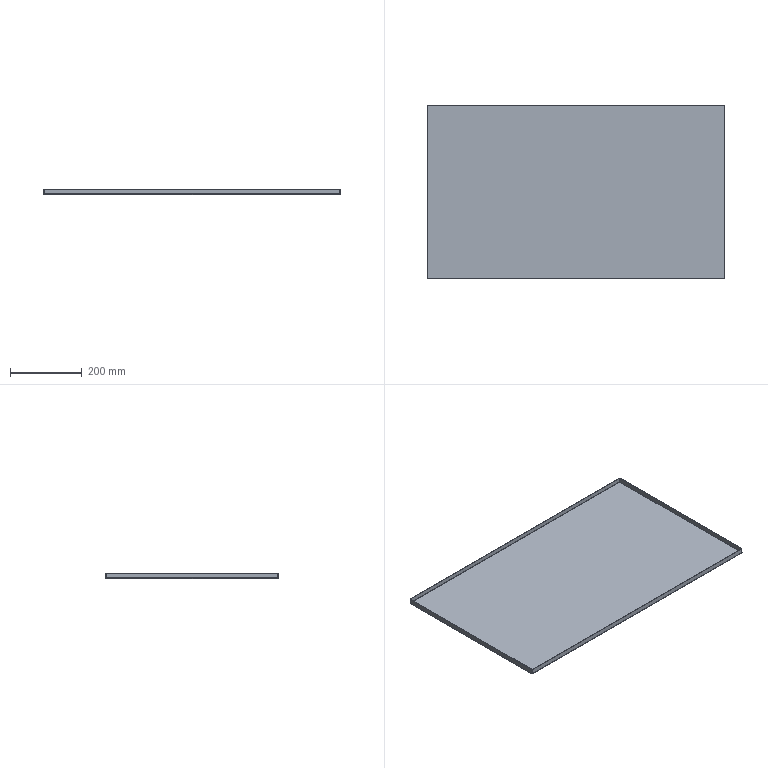Part | SolidWorks | 1 solid | 38 faces | box 830 x 485 x 15 mm | volume 870407 mm3 | plane 22 | spline 8 | cylinder 8 | commonest cylinder face diameters 0.2 x4 4.2 x4
STEP:
#1=CARTESIAN_POINT('',(412.9,-240.4,-2.));
#2=VERTEX_POINT('',#1);
#3=CARTESIAN_POINT('',(-412.9,-240.4,-2.));
#4=VERTEX_POINT('',#3);
#5=CARTESIAN_POINT('',(412.9,-240.4,-2.));
#6=DIRECTION('',(-1.,0.,0.));
#7=VECTOR('',#6,1000.);
#8=LINE('',#5,#7);
#9=EDGE_CURVE('',#2,#4,#8,.T.);
#10=ORIENTED_EDGE('',*,*,#9,.T.);
#11=CARTESIAN_POINT('',(-412.9,240.4,-2.));
#12=VERTEX_POINT('',#11);
#13=CARTESIAN_POINT('',(-412.9,-240.4,-2.));
#14=DIRECTION('',(0.,1.,0.));
#15=VECTOR('',#14,1000.);
#16=LINE('',#13,#15);
#17=EDGE_CURVE('',#4,#12,#16,.T.);
#18=ORIENTED_EDGE('',*,*,#17,.T.);
#19=CARTESIAN_POINT('',(412.9,240.4,-2.));
#20=VERTEX_POINT('',#19);
#21=CARTESIAN_POINT('',(-412.9,240.4,-2.));
#22=DIRECTION('',(1.,0.,0.));
#23=VECTOR('',#22,1000.);
#24=LINE('',#21,#23);
#25=EDGE_CURVE('',#12,#20,#24,.T.);
#26=ORIENTED_EDGE('',*,*,#25,.T.);
#27=CARTESIAN_POINT('',(412.9,240.4,-2.));
#28=DIRECTION('',(0.,-1.,0.));
#29=VECTOR('',#28,1000.);
#30=LINE('',#27,#29);
#31=EDGE_CURVE('',#20,#2,#30,.T.);
#32=ORIENTED_EDGE('',*,*,#31,.T.);
#33=EDGE_LOOP('',(#10,#18,#26,#32));
#34=FACE_OUTER_BOUND('',#33,.T.);
#35=CARTESIAN_POINT('',(0.,0.,-2.));
#36=DIRECTION('',(0.,0.,1.));
#37=DIRECTION('',(1.,0.,0.));
#38=AXIS2_PLACEMENT_3D('',#35,#36,#37);
#39=PLANE('',#38);
#40=ADVANCED_FACE('',(#34),#39,.F.);
#41=CARTESIAN_POINT('',(-412.9,-240.4,0.));
#42=VERTEX_POINT('',#41);
#43=CARTESIAN_POINT('',(-412.9,240.4,0.));
#44=VERTEX_POINT('',#43);
#45=CARTESIAN_POINT('',(-412.9,-240.4,0.));
#46=DIRECTION('',(0.,1.,0.));
#47=VECTOR('',#46,1000.);
#48=LINE('',#45,#47);
#49=EDGE_CURVE('',#42,#44,#48,.T.);
#50=ORIENTED_EDGE('',*,*,#49,.F.);
#51=CARTESIAN_POINT('',(412.9,-240.4,0.));
#52=VERTEX_POINT('',#51);
#53=CARTESIAN_POINT('',(412.9,-240.4,0.));
#54=DIRECTION('',(-1.,0.,0.));
#55=VECTOR('',#54,1000.);
#56=LINE('',#53,#55);
#57=EDGE_CURVE('',#52,#42,#56,.T.);
#58=ORIENTED_EDGE('',*,*,#57,.F.);
#59=CARTESIAN_POINT('',(412.9,240.4,0.));
#60=VERTEX_POINT('',#59);
#61=CARTESIAN_POINT('',(412.9,240.4,0.));
#62=DIRECTION('',(0.,-1.,0.));
#63=VECTOR('',#62,1000.);
#64=LINE('',#61,#63);
#65=EDGE_CURVE('',#60,#52,#64,.T.);
#66=ORIENTED_EDGE('',*,*,#65,.F.);
#67=CARTESIAN_POINT('',(-412.9,240.4,0.));
#68=DIRECTION('',(1.,0.,0.));
#69=VECTOR('',#68,1000.);
#70=LINE('',#67,#69);
#71=EDGE_CURVE('',#44,#60,#70,.T.);
#72=ORIENTED_EDGE('',*,*,#71,.F.);
#73=EDGE_LOOP('',(#50,#58,#66,#72));
#74=FACE_OUTER_BOUND('',#73,.T.);
#75=CARTESIAN_POINT('',(0.,0.,0.));
#76=DIRECTION('',(0.,0.,1.));
#77=DIRECTION('',(1.,0.,0.));
#78=AXIS2_PLACEMENT_3D('',#75,#76,#77);
#79=PLANE('',#78);
#80=ADVANCED_FACE('',(#74),#79,.T.);
#81=CARTESIAN_POINT('',(-415.,239.793,0.1));
#82=VERTEX_POINT('',#81);
#83=CARTESIAN_POINT('',(-413.,239.793,0.1));
#84=VERTEX_POINT('',#83);
#85=CARTESIAN_POINT('',(-413.,239.793,0.1));
#86=DIRECTION('',(1.,0.,0.));
#87=VECTOR('',#86,1000.);
#88=LINE('',#85,#87);
#89=EDGE_CURVE('',#82,#84,#88,.T.);
#90=ORIENTED_EDGE('',*,*,#89,.T.);
#91=CARTESIAN_POINT('',(-412.9,240.4,0.));
#92=CARTESIAN_POINT('',(-412.926,240.299,0.));
#93=CARTESIAN_POINT('',(-412.952,240.198,0.01078));
#94=CARTESIAN_POINT('',(-412.989,239.995,0.0478));
#95=CARTESIAN_POINT('',(-413.,239.894,0.07382));
#96=CARTESIAN_POINT('',(-413.,239.793,0.1));
#97=B_SPLINE_CURVE_WITH_KNOTS('',3,(#91,#92,#93,#94,#95,#96),.UNSPECIFIED.,.F.,.F.,(4,2,4),(0.,0.5,1.),.UNSPECIFIED.);
#98=EDGE_CURVE('',#44,#84,#97,.T.);
#99=ORIENTED_EDGE('',*,*,#98,.F.);
#100=CARTESIAN_POINT('',(-412.9,240.4,0.));
#101=DIRECTION('',(0.,0.,-1.));
#102=VECTOR('',#101,1000.);
#103=LINE('',#100,#102);
#104=EDGE_CURVE('',#44,#12,#103,.T.);
#105=ORIENTED_EDGE('',*,*,#104,.T.);
#106=CARTESIAN_POINT('',(-412.9,240.4,-2.));
#107=CARTESIAN_POINT('',(-413.039,240.374,-2.));
#108=CARTESIAN_POINT('',(-413.175,240.349,-1.986));
#109=CARTESIAN_POINT('',(-413.443,240.299,-1.933));
#110=CARTESIAN_POINT('',(-413.576,240.274,-1.893));
#111=CARTESIAN_POINT('',(-413.831,240.223,-1.787));
#112=CARTESIAN_POINT('',(-413.951,240.198,-1.723));
#113=CARTESIAN_POINT('',(-414.179,240.147,-1.571));
#114=CARTESIAN_POINT('',(-414.287,240.122,-1.482));
#115=CARTESIAN_POINT('',(-414.481,240.071,-1.289));
#116=CARTESIAN_POINT('',(-414.568,240.046,-1.183));
#117=CARTESIAN_POINT('',(-414.721,239.996,-0.9542));
#118=CARTESIAN_POINT('',(-414.787,239.97,-0.8315));
#119=CARTESIAN_POINT('',(-414.944,239.895,-0.4527));
#120=CARTESIAN_POINT('',(-415.,239.844,-0.1773));
#121=CARTESIAN_POINT('',(-415.,239.793,0.1));
#122=B_SPLINE_CURVE_WITH_KNOTS('',3,(#106,#107,#108,#109,#110,#111,#112,#113,#114,#115,#116,#117,#118,#119,#120,#121),.UNSPECIFIED.,.F.,.F.,(4,2,2,2,2,2,2,4),(0.,0.0004169,0.0008339,0.001251,0.001668,0.002085,0.002502,0.003336),.UNSPECIFIED.);
#123=EDGE_CURVE('',#12,#82,#122,.T.);
#124=ORIENTED_EDGE('',*,*,#123,.T.);
#125=EDGE_LOOP('',(#90,#99,#105,#124));
#126=FACE_OUTER_BOUND('',#125,.T.);
#127=CARTESIAN_POINT('',(-412.9,240.4,-2.02));
#128=CARTESIAN_POINT('',(-413.178,240.349,-2.02));
#129=CARTESIAN_POINT('',(-413.455,240.299,-1.965));
#130=CARTESIAN_POINT('',(-413.968,240.198,-1.752));
#131=CARTESIAN_POINT('',(-414.203,240.147,-1.595));
#132=CARTESIAN_POINT('',(-414.595,240.046,-1.203));
#133=CARTESIAN_POINT('',(-414.752,239.995,-0.9677));
#134=CARTESIAN_POINT('',(-414.965,239.894,-0.4549));
#135=CARTESIAN_POINT('',(-415.02,239.843,-0.1776));
#136=CARTESIAN_POINT('',(-415.02,239.793,0.1));
#137=CARTESIAN_POINT('',(-412.9,240.4,-2.));
#138=CARTESIAN_POINT('',(-413.175,240.349,-2.));
#139=CARTESIAN_POINT('',(-413.45,240.299,-1.945));
#140=CARTESIAN_POINT('',(-413.958,240.198,-1.735));
#141=CARTESIAN_POINT('',(-414.191,240.147,-1.579));
#142=CARTESIAN_POINT('',(-414.579,240.046,-1.191));
#143=CARTESIAN_POINT('',(-414.735,239.995,-0.9576));
#144=CARTESIAN_POINT('',(-414.945,239.894,-0.4497));
#145=CARTESIAN_POINT('',(-415.,239.843,-0.1749));
#146=CARTESIAN_POINT('',(-415.,239.793,0.1));
#147=CARTESIAN_POINT('',(-412.9,240.4,0.));
#148=CARTESIAN_POINT('',(-412.913,240.349,0.));
#149=CARTESIAN_POINT('',(-412.926,240.299,0.002603));
#150=CARTESIAN_POINT('',(-412.95,240.198,0.01262));
#151=CARTESIAN_POINT('',(-412.961,240.147,0.02003));
#152=CARTESIAN_POINT('',(-412.98,240.046,0.03855));
#153=CARTESIAN_POINT('',(-412.987,239.995,0.04964));
#154=CARTESIAN_POINT('',(-412.997,239.894,0.07383));
#155=CARTESIAN_POINT('',(-413.,239.843,0.08691));
#156=CARTESIAN_POINT('',(-413.,239.793,0.1));
#157=B_SPLINE_SURFACE_WITH_KNOTS('',1,3,((#127,#128,#129,#130,#131,#132,#133,#134,#135,#136),(#137,#138,#139,#140,#141,#142,#143,#144,#145,#146),(#147,#148,#149,#150,#151,#152,#153,#154,#155,#156)),.UNSPECIFIED.,.F.,.F.,.F.,(2,1,2),(4,2,2,2,4),(-0.01,0.,1.),(0.,0.25,0.5,0.75,1.),.UNSPECIFIED.);
#158=ADVANCED_FACE('',(#126),#157,.F.);
#159=CARTESIAN_POINT('',(-413.,-239.793,0.1));
#160=VERTEX_POINT('',#159);
#161=CARTESIAN_POINT('',(-413.,-239.793,0.1));
#162=CARTESIAN_POINT('',(-413.,-239.894,0.07382));
#163=CARTESIAN_POINT('',(-412.989,-239.995,0.0478));
#164=CARTESIAN_POINT('',(-412.952,-240.198,0.01078));
#165=CARTESIAN_POINT('',(-412.926,-240.299,0.));
#166=CARTESIAN_POINT('',(-412.9,-240.4,0.));
#167=B_SPLINE_CURVE_WITH_KNOTS('',3,(#161,#162,#163,#164,#165,#166),.UNSPECIFIED.,.F.,.F.,(4,2,4),(0.,0.5,1.),.UNSPECIFIED.);
#168=EDGE_CURVE('',#160,#42,#167,.T.);
#169=ORIENTED_EDGE('',*,*,#168,.F.);
#170=CARTESIAN_POINT('',(-415.,-239.793,0.1));
#171=VERTEX_POINT('',#170);
#172=CARTESIAN_POINT('',(-413.,-239.793,0.1));
#173=DIRECTION('',(1.,0.,0.));
#174=VECTOR('',#173,1000.);
#175=LINE('',#172,#174);
#176=EDGE_CURVE('',#171,#160,#175,.T.);
#177=ORIENTED_EDGE('',*,*,#176,.F.);
#178=CARTESIAN_POINT('',(-415.,-239.793,0.1));
#179=CARTESIAN_POINT('',(-415.,-239.818,-0.03865));
#180=CARTESIAN_POINT('',(-414.986,-239.844,-0.175));
#181=CARTESIAN_POINT('',(-414.933,-239.894,-0.4432));
#182=CARTESIAN_POINT('',(-414.893,-239.919,-0.5764));
#183=CARTESIAN_POINT('',(-414.787,-239.97,-0.8308));
#184=CARTESIAN_POINT('',(-414.723,-239.995,-0.9514));
#185=CARTESIAN_POINT('',(-414.571,-240.045,-1.179));
#186=CARTESIAN_POINT('',(-414.482,-240.071,-1.287));
#187=CARTESIAN_POINT('',(-414.289,-240.122,-1.481));
#188=CARTESIAN_POINT('',(-414.183,-240.147,-1.568));
#189=CARTESIAN_POINT('',(-413.954,-240.197,-1.721));
#190=CARTESIAN_POINT('',(-413.832,-240.223,-1.787));
#191=CARTESIAN_POINT('',(-413.453,-240.298,-1.944));
#192=CARTESIAN_POINT('',(-413.177,-240.349,-2.));
#193=CARTESIAN_POINT('',(-412.9,-240.4,-2.));
#194=B_SPLINE_CURVE_WITH_KNOTS('',3,(#178,#179,#180,#181,#182,#183,#184,#185,#186,#187,#188,#189,#190,#191,#192,#193),.UNSPECIFIED.,.F.,.F.,(4,2,2,2,2,2,2,4),(0.,0.0004169,0.0008339,0.001251,0.001668,0.002085,0.002502,0.003336),.UNSPECIFIED.);
#195=EDGE_CURVE('',#171,#4,#194,.T.);
#196=ORIENTED_EDGE('',*,*,#195,.T.);
#197=CARTESIAN_POINT('',(-412.9,-240.4,0.));
#198=DIRECTION('',(0.,0.,-1.));
#199=VECTOR('',#198,1000.);
#200=LINE('',#197,#199);
#201=EDGE_CURVE('',#42,#4,#200,.T.);
#202=ORIENTED_EDGE('',*,*,#201,.F.);
#203=EDGE_LOOP('',(#169,#177,#196,#202));
#204=FACE_OUTER_BOUND('',#203,.T.);
#205=CARTESIAN_POINT('',(-415.02,-239.793,0.1));
#206=CARTESIAN_POINT('',(-415.02,-239.843,-0.1776));
#207=CARTESIAN_POINT('',(-414.965,-239.894,-0.4549));
#208=CARTESIAN_POINT('',(-414.752,-239.995,-0.9677));
#209=CARTESIAN_POINT('',(-414.595,-240.046,-1.203));
#210=CARTESIAN_POINT('',(-414.203,-240.147,-1.595));
#211=CARTESIAN_POINT('',(-413.968,-240.198,-1.752));
#212=CARTESIAN_POINT('',(-413.455,-240.299,-1.965));
#213=CARTESIAN_POINT('',(-413.178,-240.349,-2.02));
#214=CARTESIAN_POINT('',(-412.9,-240.4,-2.02));
#215=CARTESIAN_POINT('',(-415.,-239.793,0.1));
#216=CARTESIAN_POINT('',(-415.,-239.843,-0.1749));
#217=CARTESIAN_POINT('',(-414.945,-239.894,-0.4497));
#218=CARTESIAN_POINT('',(-414.735,-239.995,-0.9576));
#219=CARTESIAN_POINT('',(-414.579,-240.046,-1.191));
#220=CARTESIAN_POINT('',(-414.191,-240.147,-1.579));
#221=CARTESIAN_POINT('',(-413.958,-240.198,-1.735));
#222=CARTESIAN_POINT('',(-413.45,-240.299,-1.945));
#223=CARTESIAN_POINT('',(-413.175,-240.349,-2.));
#224=CARTESIAN_POINT('',(-412.9,-240.4,-2.));
#225=CARTESIAN_POINT('',(-413.,-239.793,0.1));
#226=CARTESIAN_POINT('',(-413.,-239.843,0.08691));
#227=CARTESIAN_POINT('',(-412.997,-239.894,0.07383));
#228=CARTESIAN_POINT('',(-412.987,-239.995,0.04964));
#229=CARTESIAN_POINT('',(-412.98,-240.046,0.03855));
#230=CARTESIAN_POINT('',(-412.961,-240.147,0.02003));
#231=CARTESIAN_POINT('',(-412.95,-240.198,0.01262));
#232=CARTESIAN_POINT('',(-412.926,-240.299,0.002603));
#233=CARTESIAN_POINT('',(-412.913,-240.349,0.));
#234=CARTESIAN_POINT('',(-412.9,-240.4,0.));
#235=B_SPLINE_SURFACE_WITH_KNOTS('',1,3,((#205,#206,#207,#208,#209,#210,#211,#212,#213,#214),(#215,#216,#217,#218,#219,#220,#221,#222,#223,#224),(#225,#226,#227,#228,#229,#230,#231,#232,#233,#234)),.UNSPECIFIED.,.F.,.F.,.F.,(2,1,2),(4,2,2,2,4),(-0.01,0.,1.),(0.,0.25,0.5,0.75,1.),.UNSPECIFIED.);
#236=ADVANCED_FACE('',(#204),#235,.F.);
#237=ORIENTED_EDGE('',*,*,#17,.F.);
#238=ORIENTED_EDGE('',*,*,#195,.F.);
#239=CARTESIAN_POINT('',(-415.,242.5,0.1));
#240=DIRECTION('',(0.,1.,0.));
#241=VECTOR('',#240,1000.);
#242=LINE('',#239,#241);
#243=EDGE_CURVE('',#171,#82,#242,.T.);
#244=ORIENTED_EDGE('',*,*,#243,.T.);
#245=ORIENTED_EDGE('',*,*,#123,.F.);
#246=EDGE_LOOP('',(#237,#238,#244,#245));
#247=FACE_OUTER_BOUND('',#246,.T.);
#248=CARTESIAN_POINT('',(-412.9,-240.4,0.1));
#249=DIRECTION('',(0.,-1.,0.));
#250=DIRECTION('',(-1.,0.,0.));
#251=AXIS2_PLACEMENT_3D('',#248,#249,#250);
#252=CYLINDRICAL_SURFACE('',#251,2.1);
#253=ADVANCED_FACE('',(#247),#252,.T.);
#254=ORIENTED_EDGE('',*,*,#49,.T.);
#255=ORIENTED_EDGE('',*,*,#98,.T.);
#256=CARTESIAN_POINT('',(-413.,242.5,0.1));
#257=DIRECTION('',(0.,-1.,0.));
#258=VECTOR('',#257,1000.);
#259=LINE('',#256,#258);
#260=EDGE_CURVE('',#84,#160,#259,.T.);
#261=ORIENTED_EDGE('',*,*,#260,.T.);
#262=ORIENTED_EDGE('',*,*,#168,.T.);
#263=EDGE_LOOP('',(#254,#255,#261,#262));
#264=FACE_OUTER_BOUND('',#263,.T.);
#265=CARTESIAN_POINT('',(-412.9,-240.4,0.1));
#266=DIRECTION('',(0.,-1.,0.));
#267=DIRECTION('',(-1.,0.,0.));
#268=AXIS2_PLACEMENT_3D('',#265,#266,#267);
#269=CYLINDRICAL_SURFACE('',#268,0.1);
#270=ADVANCED_FACE('',(#264),#269,.F.);
#271=CARTESIAN_POINT('',(-415.,239.793,13.));
#272=VERTEX_POINT('',#271);
#273=CARTESIAN_POINT('',(-415.,239.793,0.));
#274=DIRECTION('',(0.,0.,1.));
#275=VECTOR('',#274,1000.);
#276=LINE('',#273,#275);
#277=EDGE_CURVE('',#82,#272,#276,.T.);
#278=ORIENTED_EDGE('',*,*,#277,.T.);
#279=CARTESIAN_POINT('',(-413.,239.793,13.));
#280=VERTEX_POINT('',#279);
#281=CARTESIAN_POINT('',(-413.,239.793,13.));
#282=DIRECTION('',(1.,0.,0.));
#283=VECTOR('',#282,1000.);
#284=LINE('',#281,#283);
#285=EDGE_CURVE('',#272,#280,#284,.T.);
#286=ORIENTED_EDGE('',*,*,#285,.T.);
#287=CARTESIAN_POINT('',(-413.,239.793,0.));
#288=DIRECTION('',(0.,0.,1.));
#289=VECTOR('',#288,1000.);
#290=LINE('',#287,#289);
#291=EDGE_CURVE('',#84,#280,#290,.T.);
#292=ORIENTED_EDGE('',*,*,#291,.F.);
#293=ORIENTED_EDGE('',*,*,#89,.F.);
#294=EDGE_LOOP('',(#278,#286,#292,#293));
#295=FACE_OUTER_BOUND('',#294,.T.);
#296=CARTESIAN_POINT('',(-413.,239.793,0.));
#297=DIRECTION('',(0.,1.,0.));
#298=DIRECTION('',(0.,0.,1.));
#299=AXIS2_PLACEMENT_3D('',#296,#297,#298);
#300=PLANE('',#299);
#301=ADVANCED_FACE('',(#295),#300,.T.);
#302=ORIENTED_EDGE('',*,*,#243,.F.);
#303=CARTESIAN_POINT('',(-415.,-239.793,13.));
#304=VERTEX_POINT('',#303);
#305=CARTESIAN_POINT('',(-415.,-239.793,0.));
#306=DIRECTION('',(0.,0.,1.));
#307=VECTOR('',#306,1000.);
#308=LINE('',#305,#307);
#309=EDGE_CURVE('',#171,#304,#308,.T.);
#310=ORIENTED_EDGE('',*,*,#309,.T.);
#311=CARTESIAN_POINT('',(-415.,0.,13.));
#312=DIRECTION('',(0.,1.,0.));
#313=VECTOR('',#312,1000.);
#314=LINE('',#311,#313);
#315=EDGE_CURVE('',#304,#272,#314,.T.);
#316=ORIENTED_EDGE('',*,*,#315,.T.);
#317=ORIENTED_EDGE('',*,*,#277,.F.);
#318=EDGE_LOOP('',(#302,#310,#316,#317));
#319=FACE_OUTER_BOUND('',#318,.T.);
#320=CARTESIAN_POINT('',(-415.,0.,0.));
#321=DIRECTION('',(1.,0.,0.));
#322=DIRECTION('',(0.,0.,-1.));
#323=AXIS2_PLACEMENT_3D('',#320,#321,#322);
#324=PLANE('',#323);
#325=ADVANCED_FACE('',(#319),#324,.F.);
#326=CARTESIAN_POINT('',(-413.,-239.793,13.));
#327=VERTEX_POINT('',#326);
#328=CARTESIAN_POINT('',(-413.,-239.793,0.));
#329=DIRECTION('',(0.,0.,1.));
#330=VECTOR('',#329,1000.);
#331=LINE('',#328,#330);
#332=EDGE_CURVE('',#160,#327,#331,.T.);
#333=ORIENTED_EDGE('',*,*,#332,.F.);
#334=ORIENTED_EDGE('',*,*,#260,.F.);
#335=ORIENTED_EDGE('',*,*,#291,.T.);
#336=CARTESIAN_POINT('',(-413.,242.5,13.));
#337=DIRECTION('',(0.,1.,0.));
#338=VECTOR('',#337,1000.);
#339=LINE('',#336,#338);
#340=EDGE_CURVE('',#327,#280,#339,.T.);
#341=ORIENTED_EDGE('',*,*,#340,.F.);
#342=EDGE_LOOP('',(#333,#334,#335,#341));
#343=FACE_OUTER_BOUND('',#342,.T.);
#344=CARTESIAN_POINT('',(-413.,0.,0.));
#345=DIRECTION('',(1.,0.,0.));
#346=DIRECTION('',(0.,0.,-1.));
#347=AXIS2_PLACEMENT_3D('',#344,#345,#346);
#348=PLANE('',#347);
#349=ADVANCED_FACE('',(#343),#348,.T.);
#350=ORIENTED_EDGE('',*,*,#315,.F.);
#351=CARTESIAN_POINT('',(-415.,-239.793,13.));
#352=DIRECTION('',(1.,0.,0.));
#353=VECTOR('',#352,1000.);
#354=LINE('',#351,#353);
#355=EDGE_CURVE('',#304,#327,#354,.T.);
#356=ORIENTED_EDGE('',*,*,#355,.T.);
#357=ORIENTED_EDGE('',*,*,#340,.T.);
#358=ORIENTED_EDGE('',*,*,#285,.F.);
#359=EDGE_LOOP('',(#350,#356,#357,#358));
#360=FACE_OUTER_BOUND('',#359,.T.);
#361=CARTESIAN_POINT('',(-415.,242.5,13.));
#362=DIRECTION('',(0.,0.,-1.));
#363=DIRECTION('',(-1.,0.,0.));
#364=AXIS2_PLACEMENT_3D('',#361,#362,#363);
#365=PLANE('',#364);
#366=ADVANCED_FACE('',(#360),#365,.F.);
#367=ORIENTED_EDGE('',*,*,#355,.F.);
#368=ORIENTED_EDGE('',*,*,#309,.F.);
#369=ORIENTED_EDGE('',*,*,#176,.T.);
#370=ORIENTED_EDGE('',*,*,#332,.T.);
#371=EDGE_LOOP('',(#367,#368,#369,#370));
#372=FACE_OUTER_BOUND('',#371,.T.);
#373=CARTESIAN_POINT('',(-413.,-239.793,0.));
#374=DIRECTION('',(0.,1.,0.));
#375=DIRECTION('',(0.,0.,1.));
#376=AXIS2_PLACEMENT_3D('',#373,#374,#375);
#377=PLANE('',#376);
#378=ADVANCED_FACE('',(#372),#377,.F.);
#379=CARTESIAN_POINT('',(412.293,242.5,0.1));
#380=VERTEX_POINT('',#379);
#381=CARTESIAN_POINT('',(412.293,240.5,0.1));
#382=VERTEX_POINT('',#381);
#383=CARTESIAN_POINT('',(412.293,240.5,0.1));
#384=DIRECTION('',(0.,-1.,0.));
#385=VECTOR('',#384,1000.);
#386=LINE('',#383,#385);
#387=EDGE_CURVE('',#380,#382,#386,.T.);
#388=ORIENTED_EDGE('',*,*,#387,.T.);
#389=CARTESIAN_POINT('',(412.9,240.4,0.));
#390=CARTESIAN_POINT('',(412.799,240.426,0.));
#391=CARTESIAN_POINT('',(412.698,240.452,0.01078));
#392=CARTESIAN_POINT('',(412.495,240.489,0.0478));
#393=CARTESIAN_POINT('',(412.394,240.5,0.07382));
#394=CARTESIAN_POINT('',(412.293,240.5,0.1));
#395=B_SPLINE_CURVE_WITH_KNOTS('',3,(#389,#390,#391,#392,#393,#394),.UNSPECIFIED.,.F.,.F.,(4,2,4),(0.,0.5,1.),.UNSPECIFIED.);
#396=EDGE_CURVE('',#60,#382,#395,.T.);
#397=ORIENTED_EDGE('',*,*,#396,.F.);
#398=CARTESIAN_POINT('',(412.9,240.4,0.));
#399=DIRECTION('',(0.,0.,-1.));
#400=VECTOR('',#399,1000.);
#401=LINE('',#398,#400);
#402=EDGE_CURVE('',#60,#20,#401,.T.);
#403=ORIENTED_EDGE('',*,*,#402,.T.);
#404=CARTESIAN_POINT('',(412.9,240.4,-2.));
#405=CARTESIAN_POINT('',(412.874,240.539,-2.));
#406=CARTESIAN_POINT('',(412.849,240.675,-1.986));
#407=CARTESIAN_POINT('',(412.799,240.943,-1.933));
#408=CARTESIAN_POINT('',(412.774,241.076,-1.893));
#409=CARTESIAN_POINT('',(412.723,241.331,-1.787));
#410=CARTESIAN_POINT('',(412.698,241.451,-1.723));
#411=CARTESIAN_POINT('',(412.647,241.679,-1.571));
#412=CARTESIAN_POINT('',(412.622,241.787,-1.482));
#413=CARTESIAN_POINT('',(412.571,241.981,-1.289));
#414=CARTESIAN_POINT('',(412.546,242.068,-1.183));
#415=CARTESIAN_POINT('',(412.496,242.221,-0.9542));
#416=CARTESIAN_POINT('',(412.47,242.287,-0.8315));
#417=CARTESIAN_POINT('',(412.395,242.444,-0.4527));
#418=CARTESIAN_POINT('',(412.344,242.5,-0.1773));
#419=CARTESIAN_POINT('',(412.293,242.5,0.1));
#420=B_SPLINE_CURVE_WITH_KNOTS('',3,(#404,#405,#406,#407,#408,#409,#410,#411,#412,#413,#414,#415,#416,#417,#418,#419),.UNSPECIFIED.,.F.,.F.,(4,2,2,2,2,2,2,4),(0.,0.0004169,0.0008339,0.001251,0.001668,0.002085,0.002502,0.003336),.UNSPECIFIED.);
#421=EDGE_CURVE('',#20,#380,#420,.T.);
#422=ORIENTED_EDGE('',*,*,#421,.T.);
#423=EDGE_LOOP('',(#388,#397,#403,#422));
#424=FACE_OUTER_BOUND('',#423,.T.);
#425=CARTESIAN_POINT('',(412.9,240.4,-2.02));
#426=CARTESIAN_POINT('',(412.849,240.678,-2.02));
#427=CARTESIAN_POINT('',(412.799,240.955,-1.965));
#428=CARTESIAN_POINT('',(412.698,241.468,-1.752));
#429=CARTESIAN_POINT('',(412.647,241.703,-1.595));
#430=CARTESIAN_POINT('',(412.546,242.095,-1.203));
#431=CARTESIAN_POINT('',(412.495,242.252,-0.9677));
#432=CARTESIAN_POINT('',(412.394,242.465,-0.4549));
#433=CARTESIAN_POINT('',(412.343,242.52,-0.1776));
#434=CARTESIAN_POINT('',(412.293,242.52,0.1));
#435=CARTESIAN_POINT('',(412.9,240.4,-2.));
#436=CARTESIAN_POINT('',(412.849,240.675,-2.));
#437=CARTESIAN_POINT('',(412.799,240.95,-1.945));
#438=CARTESIAN_POINT('',(412.698,241.458,-1.735));
#439=CARTESIAN_POINT('',(412.647,241.691,-1.579));
#440=CARTESIAN_POINT('',(412.546,242.079,-1.191));
#441=CARTESIAN_POINT('',(412.495,242.235,-0.9576));
#442=CARTESIAN_POINT('',(412.394,242.445,-0.4497));
#443=CARTESIAN_POINT('',(412.343,242.5,-0.1749));
#444=CARTESIAN_POINT('',(412.293,242.5,0.1));
#445=CARTESIAN_POINT('',(412.9,240.4,0.));
#446=CARTESIAN_POINT('',(412.849,240.413,0.));
#447=CARTESIAN_POINT('',(412.799,240.426,0.002603));
#448=CARTESIAN_POINT('',(412.698,240.45,0.01262));
#449=CARTESIAN_POINT('',(412.647,240.461,0.02003));
#450=CARTESIAN_POINT('',(412.546,240.48,0.03855));
#451=CARTESIAN_POINT('',(412.495,240.487,0.04964));
#452=CARTESIAN_POINT('',(412.394,240.497,0.07383));
#453=CARTESIAN_POINT('',(412.343,240.5,0.08691));
#454=CARTESIAN_POINT('',(412.293,240.5,0.1));
#455=B_SPLINE_SURFACE_WITH_KNOTS('',1,3,((#425,#426,#427,#428,#429,#430,#431,#432,#433,#434),(#435,#436,#437,#438,#439,#440,#441,#442,#443,#444),(#445,#446,#447,#448,#449,#450,#451,#452,#453,#454)),.UNSPECIFIED.,.F.,.F.,.F.,(2,1,2),(4,2,2,2,4),(-0.01,0.,1.),(0.,0.25,0.5,0.75,1.),.UNSPECIFIED.);
#456=ADVANCED_FACE('',(#424),#455,.F.);
#457=CARTESIAN_POINT('',(-412.293,240.5,0.1));
#458=VERTEX_POINT('',#457);
#459=CARTESIAN_POINT('',(-412.293,240.5,0.1));
#460=CARTESIAN_POINT('',(-412.394,240.5,0.07382));
#461=CARTESIAN_POINT('',(-412.495,240.489,0.0478));
#462=CARTESIAN_POINT('',(-412.698,240.452,0.01078));
#463=CARTESIAN_POINT('',(-412.799,240.426,0.));
#464=CARTESIAN_POINT('',(-412.9,240.4,0.));
#465=B_SPLINE_CURVE_WITH_KNOTS('',3,(#459,#460,#461,#462,#463,#464),.UNSPECIFIED.,.F.,.F.,(4,2,4),(0.,0.5,1.),.UNSPECIFIED.);
#466=EDGE_CURVE('',#458,#44,#465,.T.);
#467=ORIENTED_EDGE('',*,*,#466,.F.);
#468=CARTESIAN_POINT('',(-412.293,242.5,0.1));
#469=VERTEX_POINT('',#468);
#470=CARTESIAN_POINT('',(-412.293,240.5,0.1));
#471=DIRECTION('',(0.,-1.,0.));
#472=VECTOR('',#471,1000.);
#473=LINE('',#470,#472);
#474=EDGE_CURVE('',#469,#458,#473,.T.);
#475=ORIENTED_EDGE('',*,*,#474,.F.);
#476=CARTESIAN_POINT('',(-412.293,242.5,0.1));
#477=CARTESIAN_POINT('',(-412.318,242.5,-0.03865));
#478=CARTESIAN_POINT('',(-412.344,242.486,-0.175));
#479=CARTESIAN_POINT('',(-412.394,242.433,-0.4432));
#480=CARTESIAN_POINT('',(-412.419,242.393,-0.5764));
#481=CARTESIAN_POINT('',(-412.47,242.287,-0.8308));
#482=CARTESIAN_POINT('',(-412.495,242.223,-0.9514));
#483=CARTESIAN_POINT('',(-412.545,242.071,-1.179));
#484=CARTESIAN_POINT('',(-412.571,241.982,-1.287));
#485=CARTESIAN_POINT('',(-412.622,241.789,-1.481));
#486=CARTESIAN_POINT('',(-412.647,241.683,-1.568));
#487=CARTESIAN_POINT('',(-412.697,241.454,-1.721));
#488=CARTESIAN_POINT('',(-412.723,241.332,-1.787));
#489=CARTESIAN_POINT('',(-412.798,240.953,-1.944));
#490=CARTESIAN_POINT('',(-412.849,240.677,-2.));
#491=CARTESIAN_POINT('',(-412.9,240.4,-2.));
#492=B_SPLINE_CURVE_WITH_KNOTS('',3,(#476,#477,#478,#479,#480,#481,#482,#483,#484,#485,#486,#487,#488,#489,#490,#491),.UNSPECIFIED.,.F.,.F.,(4,2,2,2,2,2,2,4),(0.,0.0004169,0.0008339,0.001251,0.001668,0.002085,0.002502,0.003336),.UNSPECIFIED.);
#493=EDGE_CURVE('',#469,#12,#492,.T.);
#494=ORIENTED_EDGE('',*,*,#493,.T.);
#495=ORIENTED_EDGE('',*,*,#104,.F.);
#496=EDGE_LOOP('',(#467,#475,#494,#495));
#497=FACE_OUTER_BOUND('',#496,.T.);
#498=CARTESIAN_POINT('',(-412.293,242.52,0.1));
#499=CARTESIAN_POINT('',(-412.343,242.52,-0.1776));
#500=CARTESIAN_POINT('',(-412.394,242.465,-0.4549));
#501=CARTESIAN_POINT('',(-412.495,242.252,-0.9677));
#502=CARTESIAN_POINT('',(-412.546,242.095,-1.203));
#503=CARTESIAN_POINT('',(-412.647,241.703,-1.595));
#504=CARTESIAN_POINT('',(-412.698,241.468,-1.752));
#505=CARTESIAN_POINT('',(-412.799,240.955,-1.965));
#506=CARTESIAN_POINT('',(-412.849,240.678,-2.02));
#507=CARTESIAN_POINT('',(-412.9,240.4,-2.02));
#508=CARTESIAN_POINT('',(-412.293,242.5,0.1));
#509=CARTESIAN_POINT('',(-412.343,242.5,-0.1749));
#510=CARTESIAN_POINT('',(-412.394,242.445,-0.4497));
#511=CARTESIAN_POINT('',(-412.495,242.235,-0.9576));
#512=CARTESIAN_POINT('',(-412.546,242.079,-1.191));
#513=CARTESIAN_POINT('',(-412.647,241.691,-1.579));
#514=CARTESIAN_POINT('',(-412.698,241.458,-1.735));
#515=CARTESIAN_POINT('',(-412.799,240.95,-1.945));
#516=CARTESIAN_POINT('',(-412.849,240.675,-2.));
#517=CARTESIAN_POINT('',(-412.9,240.4,-2.));
#518=CARTESIAN_POINT('',(-412.293,240.5,0.1));
#519=CARTESIAN_POINT('',(-412.343,240.5,0.08691));
#520=CARTESIAN_POINT('',(-412.394,240.497,0.07383));
#521=CARTESIAN_POINT('',(-412.495,240.487,0.04964));
#522=CARTESIAN_POINT('',(-412.546,240.48,0.03855));
#523=CARTESIAN_POINT('',(-412.647,240.461,0.02003));
#524=CARTESIAN_POINT('',(-412.698,240.45,0.01262));
#525=CARTESIAN_POINT('',(-412.799,240.426,0.002603));
#526=CARTESIAN_POINT('',(-412.849,240.413,0.));
#527=CARTESIAN_POINT('',(-412.9,240.4,0.));
#528=B_SPLINE_SURFACE_WITH_KNOTS('',1,3,((#498,#499,#500,#501,#502,#503,#504,#505,#506,#507),(#508,#509,#510,#511,#512,#513,#514,#515,#516,#517),(#518,#519,#520,#521,#522,#523,#524,#525,#526,#527)),.UNSPECIFIED.,.F.,.F.,.F.,(2,1,2),(4,2,2,2,4),(-0.01,0.,1.),(0.,0.25,0.5,0.75,1.),.UNSPECIFIED.);
#529=ADVANCED_FACE('',(#497),#528,.F.);
#530=ORIENTED_EDGE('',*,*,#25,.F.);
#531=ORIENTED_EDGE('',*,*,#493,.F.);
#532=CARTESIAN_POINT('',(415.,242.5,0.1));
#533=DIRECTION('',(1.,0.,0.));
#534=VECTOR('',#533,1000.);
#535=LINE('',#532,#534);
#536=EDGE_CURVE('',#469,#380,#535,.T.);
#537=ORIENTED_EDGE('',*,*,#536,.T.);
#538=ORIENTED_EDGE('',*,*,#421,.F.);
#539=EDGE_LOOP('',(#530,#531,#537,#538));
#540=FACE_OUTER_BOUND('',#539,.T.);
#541=CARTESIAN_POINT('',(-412.9,240.4,0.1));
#542=DIRECTION('',(-1.,0.,0.));
#543=DIRECTION('',(0.,1.,0.));
#544=AXIS2_PLACEMENT_3D('',#541,#542,#543);
#545=CYLINDRICAL_SURFACE('',#544,2.1);
#546=ADVANCED_FACE('',(#540),#545,.T.);
#547=ORIENTED_EDGE('',*,*,#71,.T.);
#548=ORIENTED_EDGE('',*,*,#396,.T.);
#549=CARTESIAN_POINT('',(415.,240.5,0.1));
#550=DIRECTION('',(-1.,0.,0.));
#551=VECTOR('',#550,1000.);
#552=LINE('',#549,#551);
#553=EDGE_CURVE('',#382,#458,#552,.T.);
#554=ORIENTED_EDGE('',*,*,#553,.T.);
#555=ORIENTED_EDGE('',*,*,#466,.T.);
#556=EDGE_LOOP('',(#547,#548,#554,#555));
#557=FACE_OUTER_BOUND('',#556,.T.);
#558=CARTESIAN_POINT('',(-412.9,240.4,0.1));
#559=DIRECTION('',(-1.,0.,0.));
#560=DIRECTION('',(0.,1.,0.));
#561=AXIS2_PLACEMENT_3D('',#558,#559,#560);
#562=CYLINDRICAL_SURFACE('',#561,0.1);
#563=ADVANCED_FACE('',(#557),#562,.F.);
#564=CARTESIAN_POINT('',(412.293,242.5,13.));
#565=VERTEX_POINT('',#564);
#566=CARTESIAN_POINT('',(412.293,242.5,0.));
#567=DIRECTION('',(0.,0.,1.));
#568=VECTOR('',#567,1000.);
#569=LINE('',#566,#568);
#570=EDGE_CURVE('',#380,#565,#569,.T.);
#571=ORIENTED_EDGE('',*,*,#570,.T.);
#572=CARTESIAN_POINT('',(412.293,240.5,13.));
#573=VERTEX_POINT('',#572);
#574=CARTESIAN_POINT('',(412.293,240.5,13.));
#575=DIRECTION('',(0.,-1.,0.));
#576=VECTOR('',#575,1000.);
#577=LINE('',#574,#576);
#578=EDGE_CURVE('',#565,#573,#577,.T.);
#579=ORIENTED_EDGE('',*,*,#578,.T.);
#580=CARTESIAN_POINT('',(412.293,240.5,0.));
#581=DIRECTION('',(0.,0.,1.));
#582=VECTOR('',#581,1000.);
#583=LINE('',#580,#582);
#584=EDGE_CURVE('',#382,#573,#583,.T.);
#585=ORIENTED_EDGE('',*,*,#584,.F.);
#586=ORIENTED_EDGE('',*,*,#387,.F.);
#587=EDGE_LOOP('',(#571,#579,#585,#586));
#588=FACE_OUTER_BOUND('',#587,.T.);
#589=CARTESIAN_POINT('',(412.293,240.5,0.));
#590=DIRECTION('',(1.,0.,0.));
#591=DIRECTION('',(0.,0.,-1.));
#592=AXIS2_PLACEMENT_3D('',#589,#590,#591);
#593=PLANE('',#592);
#594=ADVANCED_FACE('',(#588),#593,.T.);
#595=ORIENTED_EDGE('',*,*,#536,.F.);
#596=CARTESIAN_POINT('',(-412.293,242.5,13.));
#597=VERTEX_POINT('',#596);
#598=CARTESIAN_POINT('',(-412.293,242.5,0.));
#599=DIRECTION('',(0.,0.,1.));
#600=VECTOR('',#599,1000.);
#601=LINE('',#598,#600);
#602=EDGE_CURVE('',#469,#597,#601,.T.);
#603=ORIENTED_EDGE('',*,*,#602,.T.);
#604=CARTESIAN_POINT('',(0.,242.5,13.));
#605=DIRECTION('',(1.,0.,0.));
#606=VECTOR('',#605,1000.);
#607=LINE('',#604,#606);
#608=EDGE_CURVE('',#597,#565,#607,.T.);
#609=ORIENTED_EDGE('',*,*,#608,.T.);
#610=ORIENTED_EDGE('',*,*,#570,.F.);
#611=EDGE_LOOP('',(#595,#603,#609,#610));
#612=FACE_OUTER_BOUND('',#611,.T.);
#613=CARTESIAN_POINT('',(0.,242.5,0.));
#614=DIRECTION('',(0.,-1.,0.));
#615=DIRECTION('',(0.,0.,-1.));
#616=AXIS2_PLACEMENT_3D('',#613,#614,#615);
#617=PLANE('',#616);
#618=ADVANCED_FACE('',(#612),#617,.F.);
#619=CARTESIAN_POINT('',(-412.293,240.5,13.));
#620=VERTEX_POINT('',#619);
#621=CARTESIAN_POINT('',(-412.293,240.5,0.));
#622=DIRECTION('',(0.,0.,1.));
#623=VECTOR('',#622,1000.);
#624=LINE('',#621,#623);
#625=EDGE_CURVE('',#458,#620,#624,.T.);
#626=ORIENTED_EDGE('',*,*,#625,.F.);
#627=ORIENTED_EDGE('',*,*,#553,.F.);
#628=ORIENTED_EDGE('',*,*,#584,.T.);
#629=CARTESIAN_POINT('',(415.,240.5,13.));
#630=DIRECTION('',(1.,0.,0.));
#631=VECTOR('',#630,1000.);
#632=LINE('',#629,#631);
#633=EDGE_CURVE('',#620,#573,#632,.T.);
#634=ORIENTED_EDGE('',*,*,#633,.F.);
#635=EDGE_LOOP('',(#626,#627,#628,#634));
#636=FACE_OUTER_BOUND('',#635,.T.);
#637=CARTESIAN_POINT('',(0.,240.5,0.));
#638=DIRECTION('',(0.,-1.,0.));
#639=DIRECTION('',(0.,0.,-1.));
#640=AXIS2_PLACEMENT_3D('',#637,#638,#639);
#641=PLANE('',#640);
#642=ADVANCED_FACE('',(#636),#641,.T.);
#643=ORIENTED_EDGE('',*,*,#608,.F.);
#644=CARTESIAN_POINT('',(-412.293,242.5,13.));
#645=DIRECTION('',(0.,-1.,0.));
#646=VECTOR('',#645,1000.);
#647=LINE('',#644,#646);
#648=EDGE_CURVE('',#597,#620,#647,.T.);
#649=ORIENTED_EDGE('',*,*,#648,.T.);
#650=ORIENTED_EDGE('',*,*,#633,.T.);
#651=ORIENTED_EDGE('',*,*,#578,.F.);
#652=EDGE_LOOP('',(#643,#649,#650,#651));
#653=FACE_OUTER_BOUND('',#652,.T.);
#654=CARTESIAN_POINT('',(415.,242.5,13.));
#655=DIRECTION('',(0.,0.,-1.));
#656=DIRECTION('',(0.,1.,0.));
#657=AXIS2_PLACEMENT_3D('',#654,#655,#656);
#658=PLANE('',#657);
#659=ADVANCED_FACE('',(#653),#658,.F.);
#660=ORIENTED_EDGE('',*,*,#648,.F.);
#661=ORIENTED_EDGE('',*,*,#602,.F.);
#662=ORIENTED_EDGE('',*,*,#474,.T.);
#663=ORIENTED_EDGE('',*,*,#625,.T.);
#664=EDGE_LOOP('',(#660,#661,#662,#663));
#665=FACE_OUTER_BOUND('',#664,.T.);
#666=CARTESIAN_POINT('',(-412.293,240.5,0.));
#667=DIRECTION('',(1.,0.,0.));
#668=DIRECTION('',(0.,0.,-1.));
#669=AXIS2_PLACEMENT_3D('',#666,#667,#668);
#670=PLANE('',#669);
#671=ADVANCED_FACE('',(#665),#670,.F.);
#672=CARTESIAN_POINT('',(415.,-239.793,0.1));
#673=VERTEX_POINT('',#672);
#674=CARTESIAN_POINT('',(413.,-239.793,0.1));
#675=VERTEX_POINT('',#674);
#676=CARTESIAN_POINT('',(413.,-239.793,0.1));
#677=DIRECTION('',(-1.,0.,0.));
#678=VECTOR('',#677,1000.);
#679=LINE('',#676,#678);
#680=EDGE_CURVE('',#673,#675,#679,.T.);
#681=ORIENTED_EDGE('',*,*,#680,.T.);
#682=CARTESIAN_POINT('',(412.9,-240.4,0.));
#683=CARTESIAN_POINT('',(412.926,-240.299,0.));
#684=CARTESIAN_POINT('',(412.952,-240.198,0.01078));
#685=CARTESIAN_POINT('',(412.989,-239.995,0.0478));
#686=CARTESIAN_POINT('',(413.,-239.894,0.07382));
#687=CARTESIAN_POINT('',(413.,-239.793,0.1));
#688=B_SPLINE_CURVE_WITH_KNOTS('',3,(#682,#683,#684,#685,#686,#687),.UNSPECIFIED.,.F.,.F.,(4,2,4),(0.,0.5,1.),.UNSPECIFIED.);
#689=EDGE_CURVE('',#52,#675,#688,.T.);
#690=ORIENTED_EDGE('',*,*,#689,.F.);
#691=CARTESIAN_POINT('',(412.9,-240.4,0.));
#692=DIRECTION('',(0.,0.,-1.));
#693=VECTOR('',#692,1000.);
#694=LINE('',#691,#693);
#695=EDGE_CURVE('',#52,#2,#694,.T.);
#696=ORIENTED_EDGE('',*,*,#695,.T.);
#697=CARTESIAN_POINT('',(412.9,-240.4,-2.));
#698=CARTESIAN_POINT('',(413.039,-240.374,-2.));
#699=CARTESIAN_POINT('',(413.175,-240.349,-1.986));
#700=CARTESIAN_POINT('',(413.443,-240.299,-1.933));
#701=CARTESIAN_POINT('',(413.576,-240.274,-1.893));
#702=CARTESIAN_POINT('',(413.831,-240.223,-1.787));
#703=CARTESIAN_POINT('',(413.951,-240.198,-1.723));
#704=CARTESIAN_POINT('',(414.179,-240.147,-1.571));
#705=CARTESIAN_POINT('',(414.287,-240.122,-1.482));
#706=CARTESIAN_POINT('',(414.481,-240.071,-1.289));
#707=CARTESIAN_POINT('',(414.568,-240.046,-1.183));
#708=CARTESIAN_POINT('',(414.721,-239.996,-0.9542));
#709=CARTESIAN_POINT('',(414.787,-239.97,-0.8315));
#710=CARTESIAN_POINT('',(414.944,-239.895,-0.4527));
#711=CARTESIAN_POINT('',(415.,-239.844,-0.1773));
#712=CARTESIAN_POINT('',(415.,-239.793,0.1));
#713=B_SPLINE_CURVE_WITH_KNOTS('',3,(#697,#698,#699,#700,#701,#702,#703,#704,#705,#706,#707,#708,#709,#710,#711,#712),.UNSPECIFIED.,.F.,.F.,(4,2,2,2,2,2,2,4),(0.,0.0004169,0.0008339,0.001251,0.001668,0.002085,0.002502,0.003336),.UNSPECIFIED.);
#714=EDGE_CURVE('',#2,#673,#713,.T.);
#715=ORIENTED_EDGE('',*,*,#714,.T.);
#716=EDGE_LOOP('',(#681,#690,#696,#715));
#717=FACE_OUTER_BOUND('',#716,.T.);
#718=CARTESIAN_POINT('',(412.9,-240.4,-2.02));
#719=CARTESIAN_POINT('',(413.178,-240.349,-2.02));
#720=CARTESIAN_POINT('',(413.455,-240.299,-1.965));
#721=CARTESIAN_POINT('',(413.968,-240.198,-1.752));
#722=CARTESIAN_POINT('',(414.203,-240.147,-1.595));
#723=CARTESIAN_POINT('',(414.595,-240.046,-1.203));
#724=CARTESIAN_POINT('',(414.752,-239.995,-0.9677));
#725=CARTESIAN_POINT('',(414.965,-239.894,-0.4549));
#726=CARTESIAN_POINT('',(415.02,-239.843,-0.1776));
#727=CARTESIAN_POINT('',(415.02,-239.793,0.1));
#728=CARTESIAN_POINT('',(412.9,-240.4,-2.));
#729=CARTESIAN_POINT('',(413.175,-240.349,-2.));
#730=CARTESIAN_POINT('',(413.45,-240.299,-1.945));
#731=CARTESIAN_POINT('',(413.958,-240.198,-1.735));
#732=CARTESIAN_POINT('',(414.191,-240.147,-1.579));
#733=CARTESIAN_POINT('',(414.579,-240.046,-1.191));
#734=CARTESIAN_POINT('',(414.735,-239.995,-0.9576));
#735=CARTESIAN_POINT('',(414.945,-239.894,-0.4497));
#736=CARTESIAN_POINT('',(415.,-239.843,-0.1749));
#737=CARTESIAN_POINT('',(415.,-239.793,0.1));
#738=CARTESIAN_POINT('',(412.9,-240.4,0.));
#739=CARTESIAN_POINT('',(412.913,-240.349,0.));
#740=CARTESIAN_POINT('',(412.926,-240.299,0.002603));
#741=CARTESIAN_POINT('',(412.95,-240.198,0.01262));
#742=CARTESIAN_POINT('',(412.961,-240.147,0.02003));
#743=CARTESIAN_POINT('',(412.98,-240.046,0.03855));
#744=CARTESIAN_POINT('',(412.987,-239.995,0.04964));
#745=CARTESIAN_POINT('',(412.997,-239.894,0.07383));
#746=CARTESIAN_POINT('',(413.,-239.843,0.08691));
#747=CARTESIAN_POINT('',(413.,-239.793,0.1));
#748=B_SPLINE_SURFACE_WITH_KNOTS('',1,3,((#718,#719,#720,#721,#722,#723,#724,#725,#726,#727),(#728,#729,#730,#731,#732,#733,#734,#735,#736,#737),(#738,#739,#740,#741,#742,#743,#744,#745,#746,#747)),.UNSPECIFIED.,.F.,.F.,.F.,(2,1,2),(4,2,2,2,4),(-0.01,0.,1.),(0.,0.25,0.5,0.75,1.),.UNSPECIFIED.);
#749=ADVANCED_FACE('',(#717),#748,.F.);
#750=CARTESIAN_POINT('',(413.,239.793,0.1));
#751=VERTEX_POINT('',#750);
#752=CARTESIAN_POINT('',(413.,239.793,0.1));
#753=CARTESIAN_POINT('',(413.,239.894,0.07382));
#754=CARTESIAN_POINT('',(412.989,239.995,0.0478));
#755=CARTESIAN_POINT('',(412.952,240.198,0.01078));
#756=CARTESIAN_POINT('',(412.926,240.299,0.));
#757=CARTESIAN_POINT('',(412.9,240.4,0.));
#758=B_SPLINE_CURVE_WITH_KNOTS('',3,(#752,#753,#754,#755,#756,#757),.UNSPECIFIED.,.F.,.F.,(4,2,4),(0.,0.5,1.),.UNSPECIFIED.);
#759=EDGE_CURVE('',#751,#60,#758,.T.);
#760=ORIENTED_EDGE('',*,*,#759,.F.);
#761=CARTESIAN_POINT('',(415.,239.793,0.1));
#762=VERTEX_POINT('',#761);
#763=CARTESIAN_POINT('',(413.,239.793,0.1));
#764=DIRECTION('',(-1.,0.,0.));
#765=VECTOR('',#764,1000.);
#766=LINE('',#763,#765);
#767=EDGE_CURVE('',#762,#751,#766,.T.);
#768=ORIENTED_EDGE('',*,*,#767,.F.);
#769=CARTESIAN_POINT('',(415.,239.793,0.1));
#770=CARTESIAN_POINT('',(415.,239.818,-0.03865));
#771=CARTESIAN_POINT('',(414.986,239.844,-0.175));
#772=CARTESIAN_POINT('',(414.933,239.894,-0.4432));
#773=CARTESIAN_POINT('',(414.893,239.919,-0.5764));
#774=CARTESIAN_POINT('',(414.787,239.97,-0.8308));
#775=CARTESIAN_POINT('',(414.723,239.995,-0.9514));
#776=CARTESIAN_POINT('',(414.571,240.045,-1.179));
#777=CARTESIAN_POINT('',(414.482,240.071,-1.287));
#778=CARTESIAN_POINT('',(414.289,240.122,-1.481));
#779=CARTESIAN_POINT('',(414.183,240.147,-1.568));
#780=CARTESIAN_POINT('',(413.954,240.197,-1.721));
#781=CARTESIAN_POINT('',(413.832,240.223,-1.787));
#782=CARTESIAN_POINT('',(413.453,240.298,-1.944));
#783=CARTESIAN_POINT('',(413.177,240.349,-2.));
#784=CARTESIAN_POINT('',(412.9,240.4,-2.));
#785=B_SPLINE_CURVE_WITH_KNOTS('',3,(#769,#770,#771,#772,#773,#774,#775,#776,#777,#778,#779,#780,#781,#782,#783,#784),.UNSPECIFIED.,.F.,.F.,(4,2,2,2,2,2,2,4),(0.,0.0004169,0.0008339,0.001251,0.001668,0.002085,0.002502,0.003336),.UNSPECIFIED.);
#786=EDGE_CURVE('',#762,#20,#785,.T.);
#787=ORIENTED_EDGE('',*,*,#786,.T.);
#788=ORIENTED_EDGE('',*,*,#402,.F.);
#789=EDGE_LOOP('',(#760,#768,#787,#788));
#790=FACE_OUTER_BOUND('',#789,.T.);
#791=CARTESIAN_POINT('',(415.02,239.793,0.1));
#792=CARTESIAN_POINT('',(415.02,239.843,-0.1776));
#793=CARTESIAN_POINT('',(414.965,239.894,-0.4549));
#794=CARTESIAN_POINT('',(414.752,239.995,-0.9677));
#795=CARTESIAN_POINT('',(414.595,240.046,-1.203));
#796=CARTESIAN_POINT('',(414.203,240.147,-1.595));
#797=CARTESIAN_POINT('',(413.968,240.198,-1.752));
#798=CARTESIAN_POINT('',(413.455,240.299,-1.965));
#799=CARTESIAN_POINT('',(413.178,240.349,-2.02));
#800=CARTESIAN_POINT('',(412.9,240.4,-2.02));
#801=CARTESIAN_POINT('',(415.,239.793,0.1));
#802=CARTESIAN_POINT('',(415.,239.843,-0.1749));
#803=CARTESIAN_POINT('',(414.945,239.894,-0.4497));
#804=CARTESIAN_POINT('',(414.735,239.995,-0.9576));
#805=CARTESIAN_POINT('',(414.579,240.046,-1.191));
#806=CARTESIAN_POINT('',(414.191,240.147,-1.579));
#807=CARTESIAN_POINT('',(413.958,240.198,-1.735));
#808=CARTESIAN_POINT('',(413.45,240.299,-1.945));
#809=CARTESIAN_POINT('',(413.175,240.349,-2.));
#810=CARTESIAN_POINT('',(412.9,240.4,-2.));
#811=CARTESIAN_POINT('',(413.,239.793,0.1));
#812=CARTESIAN_POINT('',(413.,239.843,0.08691));
#813=CARTESIAN_POINT('',(412.997,239.894,0.07383));
#814=CARTESIAN_POINT('',(412.987,239.995,0.04964));
#815=CARTESIAN_POINT('',(412.98,240.046,0.03855));
#816=CARTESIAN_POINT('',(412.961,240.147,0.02003));
#817=CARTESIAN_POINT('',(412.95,240.198,0.01262));
#818=CARTESIAN_POINT('',(412.926,240.299,0.002603));
#819=CARTESIAN_POINT('',(412.913,240.349,0.));
#820=CARTESIAN_POINT('',(412.9,240.4,0.));
#821=B_SPLINE_SURFACE_WITH_KNOTS('',1,3,((#791,#792,#793,#794,#795,#796,#797,#798,#799,#800),(#801,#802,#803,#804,#805,#806,#807,#808,#809,#810),(#811,#812,#813,#814,#815,#816,#817,#818,#819,#820)),.UNSPECIFIED.,.F.,.F.,.F.,(2,1,2),(4,2,2,2,4),(-0.01,0.,1.),(0.,0.25,0.5,0.75,1.),.UNSPECIFIED.);
#822=ADVANCED_FACE('',(#790),#821,.F.);
#823=ORIENTED_EDGE('',*,*,#31,.F.);
#824=ORIENTED_EDGE('',*,*,#786,.F.);
#825=CARTESIAN_POINT('',(415.,-242.5,0.1));
#826=DIRECTION('',(0.,-1.,0.));
#827=VECTOR('',#826,1000.);
#828=LINE('',#825,#827);
#829=EDGE_CURVE('',#762,#673,#828,.T.);
#830=ORIENTED_EDGE('',*,*,#829,.T.);
#831=ORIENTED_EDGE('',*,*,#714,.F.);
#832=EDGE_LOOP('',(#823,#824,#830,#831));
#833=FACE_OUTER_BOUND('',#832,.T.);
#834=CARTESIAN_POINT('',(412.9,240.4,0.1));
#835=DIRECTION('',(0.,1.,0.));
#836=DIRECTION('',(1.,0.,0.));
#837=AXIS2_PLACEMENT_3D('',#834,#835,#836);
#838=CYLINDRICAL_SURFACE('',#837,2.1);
#839=ADVANCED_FACE('',(#833),#838,.T.);
#840=ORIENTED_EDGE('',*,*,#65,.T.);
#841=ORIENTED_EDGE('',*,*,#689,.T.);
#842=CARTESIAN_POINT('',(413.,-242.5,0.1));
#843=DIRECTION('',(0.,1.,0.));
#844=VECTOR('',#843,1000.);
#845=LINE('',#842,#844);
#846=EDGE_CURVE('',#675,#751,#845,.T.);
#847=ORIENTED_EDGE('',*,*,#846,.T.);
#848=ORIENTED_EDGE('',*,*,#759,.T.);
#849=EDGE_LOOP('',(#840,#841,#847,#848));
#850=FACE_OUTER_BOUND('',#849,.T.);
#851=CARTESIAN_POINT('',(412.9,240.4,0.1));
#852=DIRECTION('',(0.,1.,0.));
#853=DIRECTION('',(1.,0.,0.));
#854=AXIS2_PLACEMENT_3D('',#851,#852,#853);
#855=CYLINDRICAL_SURFACE('',#854,0.1);
#856=ADVANCED_FACE('',(#850),#855,.F.);
#857=CARTESIAN_POINT('',(415.,-239.793,13.));
#858=VERTEX_POINT('',#857);
#859=CARTESIAN_POINT('',(415.,-239.793,0.));
#860=DIRECTION('',(0.,0.,1.));
#861=VECTOR('',#860,1000.);
#862=LINE('',#859,#861);
#863=EDGE_CURVE('',#673,#858,#862,.T.);
#864=ORIENTED_EDGE('',*,*,#863,.T.);
#865=CARTESIAN_POINT('',(413.,-239.793,13.));
#866=VERTEX_POINT('',#865);
#867=CARTESIAN_POINT('',(413.,-239.793,13.));
#868=DIRECTION('',(-1.,0.,0.));
#869=VECTOR('',#868,1000.);
#870=LINE('',#867,#869);
#871=EDGE_CURVE('',#858,#866,#870,.T.);
#872=ORIENTED_EDGE('',*,*,#871,.T.);
#873=CARTESIAN_POINT('',(413.,-239.793,0.));
#874=DIRECTION('',(0.,0.,1.));
#875=VECTOR('',#874,1000.);
#876=LINE('',#873,#875);
#877=EDGE_CURVE('',#675,#866,#876,.T.);
#878=ORIENTED_EDGE('',*,*,#877,.F.);
#879=ORIENTED_EDGE('',*,*,#680,.F.);
#880=EDGE_LOOP('',(#864,#872,#878,#879));
#881=FACE_OUTER_BOUND('',#880,.T.);
#882=CARTESIAN_POINT('',(413.,-239.793,0.));
#883=DIRECTION('',(0.,-1.,0.));
#884=DIRECTION('',(0.,0.,-1.));
#885=AXIS2_PLACEMENT_3D('',#882,#883,#884);
#886=PLANE('',#885);
#887=ADVANCED_FACE('',(#881),#886,.T.);
#888=ORIENTED_EDGE('',*,*,#829,.F.);
#889=CARTESIAN_POINT('',(415.,239.793,13.));
#890=VERTEX_POINT('',#889);
#891=CARTESIAN_POINT('',(415.,239.793,0.));
#892=DIRECTION('',(0.,0.,1.));
#893=VECTOR('',#892,1000.);
#894=LINE('',#891,#893);
#895=EDGE_CURVE('',#762,#890,#894,.T.);
#896=ORIENTED_EDGE('',*,*,#895,.T.);
#897=CARTESIAN_POINT('',(415.,0.,13.));
#898=DIRECTION('',(0.,-1.,0.));
#899=VECTOR('',#898,1000.);
#900=LINE('',#897,#899);
#901=EDGE_CURVE('',#890,#858,#900,.T.);
#902=ORIENTED_EDGE('',*,*,#901,.T.);
#903=ORIENTED_EDGE('',*,*,#863,.F.);
#904=EDGE_LOOP('',(#888,#896,#902,#903));
#905=FACE_OUTER_BOUND('',#904,.T.);
#906=CARTESIAN_POINT('',(415.,0.,0.));
#907=DIRECTION('',(-1.,0.,0.));
#908=DIRECTION('',(0.,0.,1.));
#909=AXIS2_PLACEMENT_3D('',#906,#907,#908);
#910=PLANE('',#909);
#911=ADVANCED_FACE('',(#905),#910,.F.);
#912=CARTESIAN_POINT('',(413.,239.793,13.));
#913=VERTEX_POINT('',#912);
#914=CARTESIAN_POINT('',(413.,239.793,0.));
#915=DIRECTION('',(0.,0.,1.));
#916=VECTOR('',#915,1000.);
#917=LINE('',#914,#916);
#918=EDGE_CURVE('',#751,#913,#917,.T.);
#919=ORIENTED_EDGE('',*,*,#918,.F.);
#920=ORIENTED_EDGE('',*,*,#846,.F.);
#921=ORIENTED_EDGE('',*,*,#877,.T.);
#922=CARTESIAN_POINT('',(413.,-242.5,13.));
#923=DIRECTION('',(0.,-1.,0.));
#924=VECTOR('',#923,1000.);
#925=LINE('',#922,#924);
#926=EDGE_CURVE('',#913,#866,#925,.T.);
#927=ORIENTED_EDGE('',*,*,#926,.F.);
#928=EDGE_LOOP('',(#919,#920,#921,#927));
#929=FACE_OUTER_BOUND('',#928,.T.);
#930=CARTESIAN_POINT('',(413.,0.,0.));
#931=DIRECTION('',(-1.,0.,0.));
#932=DIRECTION('',(0.,0.,1.));
#933=AXIS2_PLACEMENT_3D('',#930,#931,#932);
#934=PLANE('',#933);
#935=ADVANCED_FACE('',(#929),#934,.T.);
#936=ORIENTED_EDGE('',*,*,#901,.F.);
#937=CARTESIAN_POINT('',(415.,239.793,13.));
#938=DIRECTION('',(-1.,0.,0.));
#939=VECTOR('',#938,1000.);
#940=LINE('',#937,#939);
#941=EDGE_CURVE('',#890,#913,#940,.T.);
#942=ORIENTED_EDGE('',*,*,#941,.T.);
#943=ORIENTED_EDGE('',*,*,#926,.T.);
#944=ORIENTED_EDGE('',*,*,#871,.F.);
#945=EDGE_LOOP('',(#936,#942,#943,#944));
#946=FACE_OUTER_BOUND('',#945,.T.);
#947=CARTESIAN_POINT('',(415.,-242.5,13.));
#948=DIRECTION('',(0.,0.,-1.));
#949=DIRECTION('',(-1.,0.,0.));
#950=AXIS2_PLACEMENT_3D('',#947,#948,#949);
#951=PLANE('',#950);
#952=ADVANCED_FACE('',(#946),#951,.F.);
#953=ORIENTED_EDGE('',*,*,#941,.F.);
#954=ORIENTED_EDGE('',*,*,#895,.F.);
#955=ORIENTED_EDGE('',*,*,#767,.T.);
#956=ORIENTED_EDGE('',*,*,#918,.T.);
#957=EDGE_LOOP('',(#953,#954,#955,#956));
#958=FACE_OUTER_BOUND('',#957,.T.);
#959=CARTESIAN_POINT('',(413.,239.793,0.));
#960=DIRECTION('',(0.,-1.,0.));
#961=DIRECTION('',(0.,0.,-1.));
#962=AXIS2_PLACEMENT_3D('',#959,#960,#961);
#963=PLANE('',#962);
#964=ADVANCED_FACE('',(#958),#963,.F.);
#965=CARTESIAN_POINT('',(-412.293,-242.5,0.1));
#966=VERTEX_POINT('',#965);
#967=CARTESIAN_POINT('',(-412.293,-240.5,0.1));
#968=VERTEX_POINT('',#967);
#969=CARTESIAN_POINT('',(-412.293,-240.5,0.1));
#970=DIRECTION('',(0.,1.,0.));
#971=VECTOR('',#970,1000.);
#972=LINE('',#969,#971);
#973=EDGE_CURVE('',#966,#968,#972,.T.);
#974=ORIENTED_EDGE('',*,*,#973,.T.);
#975=CARTESIAN_POINT('',(-412.9,-240.4,0.));
#976=CARTESIAN_POINT('',(-412.799,-240.426,0.));
#977=CARTESIAN_POINT('',(-412.698,-240.452,0.01078));
#978=CARTESIAN_POINT('',(-412.495,-240.489,0.0478));
#979=CARTESIAN_POINT('',(-412.394,-240.5,0.07382));
#980=CARTESIAN_POINT('',(-412.293,-240.5,0.1));
#981=B_SPLINE_CURVE_WITH_KNOTS('',3,(#975,#976,#977,#978,#979,#980),.UNSPECIFIED.,.F.,.F.,(4,2,4),(0.,0.5,1.),.UNSPECIFIED.);
#982=EDGE_CURVE('',#42,#968,#981,.T.);
#983=ORIENTED_EDGE('',*,*,#982,.F.);
#984=ORIENTED_EDGE('',*,*,#201,.T.);
#985=CARTESIAN_POINT('',(-412.9,-240.4,-2.));
#986=CARTESIAN_POINT('',(-412.874,-240.539,-2.));
#987=CARTESIAN_POINT('',(-412.849,-240.675,-1.986));
#988=CARTESIAN_POINT('',(-412.799,-240.943,-1.933));
#989=CARTESIAN_POINT('',(-412.774,-241.076,-1.893));
#990=CARTESIAN_POINT('',(-412.723,-241.331,-1.787));
#991=CARTESIAN_POINT('',(-412.698,-241.451,-1.723));
#992=CARTESIAN_POINT('',(-412.647,-241.679,-1.571));
#993=CARTESIAN_POINT('',(-412.622,-241.787,-1.482));
#994=CARTESIAN_POINT('',(-412.571,-241.981,-1.289));
#995=CARTESIAN_POINT('',(-412.546,-242.068,-1.183));
#996=CARTESIAN_POINT('',(-412.496,-242.221,-0.9542));
#997=CARTESIAN_POINT('',(-412.47,-242.287,-0.8315));
#998=CARTESIAN_POINT('',(-412.395,-242.444,-0.4527));
#999=CARTESIAN_POINT('',(-412.344,-242.5,-0.1773));
#1000=CARTESIAN_POINT('',(-412.293,-242.5,0.1));
#1001=B_SPLINE_CURVE_WITH_KNOTS('',3,(#985,#986,#987,#988,#989,#990,#991,#992,#993,#994,#995,#996,#997,#998,#999,#1000),.UNSPECIFIED.,.F.,.F.,(4,2,2,2,2,2,2,4),(0.,0.0004169,0.0008339,0.001251,0.001668,0.002085,0.002502,0.003336),.UNSPECIFIED.);
#1002=EDGE_CURVE('',#4,#966,#1001,.T.);
#1003=ORIENTED_EDGE('',*,*,#1002,.T.);
#1004=EDGE_LOOP('',(#974,#983,#984,#1003));
#1005=FACE_OUTER_BOUND('',#1004,.T.);
#1006=CARTESIAN_POINT('',(-412.9,-240.4,-2.02));
#1007=CARTESIAN_POINT('',(-412.849,-240.678,-2.02));
#1008=CARTESIAN_POINT('',(-412.799,-240.955,-1.965));
#1009=CARTESIAN_POINT('',(-412.698,-241.468,-1.752));
#1010=CARTESIAN_POINT('',(-412.647,-241.703,-1.595));
#1011=CARTESIAN_POINT('',(-412.546,-242.095,-1.203));
#1012=CARTESIAN_POINT('',(-412.495,-242.252,-0.9677));
#1013=CARTESIAN_POINT('',(-412.394,-242.465,-0.4549));
#1014=CARTESIAN_POINT('',(-412.343,-242.52,-0.1776));
#1015=CARTESIAN_POINT('',(-412.293,-242.52,0.1));
#1016=CARTESIAN_POINT('',(-412.9,-240.4,-2.));
#1017=CARTESIAN_POINT('',(-412.849,-240.675,-2.));
#1018=CARTESIAN_POINT('',(-412.799,-240.95,-1.945));
#1019=CARTESIAN_POINT('',(-412.698,-241.458,-1.735));
#1020=CARTESIAN_POINT('',(-412.647,-241.691,-1.579));
#1021=CARTESIAN_POINT('',(-412.546,-242.079,-1.191));
#1022=CARTESIAN_POINT('',(-412.495,-242.235,-0.9576));
#1023=CARTESIAN_POINT('',(-412.394,-242.445,-0.4497));
#1024=CARTESIAN_POINT('',(-412.343,-242.5,-0.1749));
#1025=CARTESIAN_POINT('',(-412.293,-242.5,0.1));
#1026=CARTESIAN_POINT('',(-412.9,-240.4,0.));
#1027=CARTESIAN_POINT('',(-412.849,-240.413,0.));
#1028=CARTESIAN_POINT('',(-412.799,-240.426,0.002603));
#1029=CARTESIAN_POINT('',(-412.698,-240.45,0.01262));
#1030=CARTESIAN_POINT('',(-412.647,-240.461,0.02003));
#1031=CARTESIAN_POINT('',(-412.546,-240.48,0.03855));
#1032=CARTESIAN_POINT('',(-412.495,-240.487,0.04964));
#1033=CARTESIAN_POINT('',(-412.394,-240.497,0.07383));
#1034=CARTESIAN_POINT('',(-412.343,-240.5,0.08691));
#1035=CARTESIAN_POINT('',(-412.293,-240.5,0.1));
#1036=B_SPLINE_SURFACE_WITH_KNOTS('',1,3,((#1006,#1007,#1008,#1009,#1010,#1011,#1012,#1013,#1014,#1015),(#1016,#1017,#1018,#1019,#1020,#1021,#1022,#1023,#1024,#1025),(#1026,#1027,#1028,#1029,#1030,#1031,#1032,#1033,#1034,#1035)),.UNSPECIFIED.,.F.,.F.,.F.,(2,1,2),(4,2,2,2,4),(-0.01,0.,1.),(0.,0.25,0.5,0.75,1.),.UNSPECIFIED.);
#1037=ADVANCED_FACE('',(#1005),#1036,.F.);
#1038=CARTESIAN_POINT('',(412.293,-240.5,0.1));
#1039=VERTEX_POINT('',#1038);
#1040=CARTESIAN_POINT('',(412.293,-240.5,0.1));
#1041=CARTESIAN_POINT('',(412.394,-240.5,0.07382));
#1042=CARTESIAN_POINT('',(412.495,-240.489,0.0478));
#1043=CARTESIAN_POINT('',(412.698,-240.452,0.01078));
#1044=CARTESIAN_POINT('',(412.799,-240.426,0.));
#1045=CARTESIAN_POINT('',(412.9,-240.4,0.));
#1046=B_SPLINE_CURVE_WITH_KNOTS('',3,(#1040,#1041,#1042,#1043,#1044,#1045),.UNSPECIFIED.,.F.,.F.,(4,2,4),(0.,0.5,1.),.UNSPECIFIED.);
#1047=EDGE_CURVE('',#1039,#52,#1046,.T.);
#1048=ORIENTED_EDGE('',*,*,#1047,.F.);
#1049=CARTESIAN_POINT('',(412.293,-242.5,0.1));
#1050=VERTEX_POINT('',#1049);
#1051=CARTESIAN_POINT('',(412.293,-240.5,0.1));
#1052=DIRECTION('',(0.,1.,0.));
#1053=VECTOR('',#1052,1000.);
#1054=LINE('',#1051,#1053);
#1055=EDGE_CURVE('',#1050,#1039,#1054,.T.);
#1056=ORIENTED_EDGE('',*,*,#1055,.F.);
#1057=CARTESIAN_POINT('',(412.293,-242.5,0.1));
#1058=CARTESIAN_POINT('',(412.318,-242.5,-0.03865));
#1059=CARTESIAN_POINT('',(412.344,-242.486,-0.175));
#1060=CARTESIAN_POINT('',(412.394,-242.433,-0.4432));
#1061=CARTESIAN_POINT('',(412.419,-242.393,-0.5764));
#1062=CARTESIAN_POINT('',(412.47,-242.287,-0.8308));
#1063=CARTESIAN_POINT('',(412.495,-242.223,-0.9514));
#1064=CARTESIAN_POINT('',(412.545,-242.071,-1.179));
#1065=CARTESIAN_POINT('',(412.571,-241.982,-1.287));
#1066=CARTESIAN_POINT('',(412.622,-241.789,-1.481));
#1067=CARTESIAN_POINT('',(412.647,-241.683,-1.568));
#1068=CARTESIAN_POINT('',(412.697,-241.454,-1.721));
#1069=CARTESIAN_POINT('',(412.723,-241.332,-1.787));
#1070=CARTESIAN_POINT('',(412.798,-240.953,-1.944));
#1071=CARTESIAN_POINT('',(412.849,-240.677,-2.));
#1072=CARTESIAN_POINT('',(412.9,-240.4,-2.));
#1073=B_SPLINE_CURVE_WITH_KNOTS('',3,(#1057,#1058,#1059,#1060,#1061,#1062,#1063,#1064,#1065,#1066,#1067,#1068,#1069,#1070,#1071,#1072),.UNSPECIFIED.,.F.,.F.,(4,2,2,2,2,2,2,4),(0.,0.0004169,0.0008339,0.001251,0.001668,0.002085,0.002502,0.003336),.UNSPECIFIED.);
#1074=EDGE_CURVE('',#1050,#2,#1073,.T.);
#1075=ORIENTED_EDGE('',*,*,#1074,.T.);
#1076=ORIENTED_EDGE('',*,*,#695,.F.);
#1077=EDGE_LOOP('',(#1048,#1056,#1075,#1076));
#1078=FACE_OUTER_BOUND('',#1077,.T.);
#1079=CARTESIAN_POINT('',(412.293,-242.52,0.1));
#1080=CARTESIAN_POINT('',(412.343,-242.52,-0.1776));
#1081=CARTESIAN_POINT('',(412.394,-242.465,-0.4549));
#1082=CARTESIAN_POINT('',(412.495,-242.252,-0.9677));
#1083=CARTESIAN_POINT('',(412.546,-242.095,-1.203));
#1084=CARTESIAN_POINT('',(412.647,-241.703,-1.595));
#1085=CARTESIAN_POINT('',(412.698,-241.468,-1.752));
#1086=CARTESIAN_POINT('',(412.799,-240.955,-1.965));
#1087=CARTESIAN_POINT('',(412.849,-240.678,-2.02));
#1088=CARTESIAN_POINT('',(412.9,-240.4,-2.02));
#1089=CARTESIAN_POINT('',(412.293,-242.5,0.1));
#1090=CARTESIAN_POINT('',(412.343,-242.5,-0.1749));
#1091=CARTESIAN_POINT('',(412.394,-242.445,-0.4497));
#1092=CARTESIAN_POINT('',(412.495,-242.235,-0.9576));
#1093=CARTESIAN_POINT('',(412.546,-242.079,-1.191));
#1094=CARTESIAN_POINT('',(412.647,-241.691,-1.579));
#1095=CARTESIAN_POINT('',(412.698,-241.458,-1.735));
#1096=CARTESIAN_POINT('',(412.799,-240.95,-1.945));
#1097=CARTESIAN_POINT('',(412.849,-240.675,-2.));
#1098=CARTESIAN_POINT('',(412.9,-240.4,-2.));
#1099=CARTESIAN_POINT('',(412.293,-240.5,0.1));
#1100=CARTESIAN_POINT('',(412.343,-240.5,0.08691));
#1101=CARTESIAN_POINT('',(412.394,-240.497,0.07383));
#1102=CARTESIAN_POINT('',(412.495,-240.487,0.04964));
#1103=CARTESIAN_POINT('',(412.546,-240.48,0.03855));
#1104=CARTESIAN_POINT('',(412.647,-240.461,0.02003));
#1105=CARTESIAN_POINT('',(412.698,-240.45,0.01262));
#1106=CARTESIAN_POINT('',(412.799,-240.426,0.002603));
#1107=CARTESIAN_POINT('',(412.849,-240.413,0.));
#1108=CARTESIAN_POINT('',(412.9,-240.4,0.));
#1109=B_SPLINE_SURFACE_WITH_KNOTS('',1,3,((#1079,#1080,#1081,#1082,#1083,#1084,#1085,#1086,#1087,#1088),(#1089,#1090,#1091,#1092,#1093,#1094,#1095,#1096,#1097,#1098),(#1099,#1100,#1101,#1102,#1103,#1104,#1105,#1106,#1107,#1108)),.UNSPECIFIED.,.F.,.F.,.F.,(2,1,2),(4,2,2,2,4),(-0.01,0.,1.),(0.,0.25,0.5,0.75,1.),.UNSPECIFIED.);
#1110=ADVANCED_FACE('',(#1078),#1109,.F.);
#1111=ORIENTED_EDGE('',*,*,#9,.F.);
#1112=ORIENTED_EDGE('',*,*,#1074,.F.);
#1113=CARTESIAN_POINT('',(-415.,-242.5,0.1));
#1114=DIRECTION('',(-1.,0.,0.));
#1115=VECTOR('',#1114,1000.);
#1116=LINE('',#1113,#1115);
#1117=EDGE_CURVE('',#1050,#966,#1116,.T.);
#1118=ORIENTED_EDGE('',*,*,#1117,.T.);
#1119=ORIENTED_EDGE('',*,*,#1002,.F.);
#1120=EDGE_LOOP('',(#1111,#1112,#1118,#1119));
#1121=FACE_OUTER_BOUND('',#1120,.T.);
#1122=CARTESIAN_POINT('',(412.9,-240.4,0.1));
#1123=DIRECTION('',(1.,0.,0.));
#1124=DIRECTION('',(0.,-1.,0.));
#1125=AXIS2_PLACEMENT_3D('',#1122,#1123,#1124);
#1126=CYLINDRICAL_SURFACE('',#1125,2.1);
#1127=ADVANCED_FACE('',(#1121),#1126,.T.);
#1128=ORIENTED_EDGE('',*,*,#57,.T.);
#1129=ORIENTED_EDGE('',*,*,#982,.T.);
#1130=CARTESIAN_POINT('',(-415.,-240.5,0.1));
#1131=DIRECTION('',(1.,0.,0.));
#1132=VECTOR('',#1131,1000.);
#1133=LINE('',#1130,#1132);
#1134=EDGE_CURVE('',#968,#1039,#1133,.T.);
#1135=ORIENTED_EDGE('',*,*,#1134,.T.);
#1136=ORIENTED_EDGE('',*,*,#1047,.T.);
#1137=EDGE_LOOP('',(#1128,#1129,#1135,#1136));
#1138=FACE_OUTER_BOUND('',#1137,.T.);
#1139=CARTESIAN_POINT('',(412.9,-240.4,0.1));
#1140=DIRECTION('',(1.,0.,0.));
#1141=DIRECTION('',(0.,-1.,0.));
#1142=AXIS2_PLACEMENT_3D('',#1139,#1140,#1141);
#1143=CYLINDRICAL_SURFACE('',#1142,0.1);
#1144=ADVANCED_FACE('',(#1138),#1143,.F.);
#1145=CARTESIAN_POINT('',(-412.293,-242.5,13.));
#1146=VERTEX_POINT('',#1145);
#1147=CARTESIAN_POINT('',(-412.293,-242.5,0.));
#1148=DIRECTION('',(0.,0.,1.));
#1149=VECTOR('',#1148,1000.);
#1150=LINE('',#1147,#1149);
#1151=EDGE_CURVE('',#966,#1146,#1150,.T.);
#1152=ORIENTED_EDGE('',*,*,#1151,.T.);
#1153=CARTESIAN_POINT('',(-412.293,-240.5,13.));
#1154=VERTEX_POINT('',#1153);
#1155=CARTESIAN_POINT('',(-412.293,-240.5,13.));
#1156=DIRECTION('',(0.,1.,0.));
#1157=VECTOR('',#1156,1000.);
#1158=LINE('',#1155,#1157);
#1159=EDGE_CURVE('',#1146,#1154,#1158,.T.);
#1160=ORIENTED_EDGE('',*,*,#1159,.T.);
#1161=CARTESIAN_POINT('',(-412.293,-240.5,0.));
#1162=DIRECTION('',(0.,0.,1.));
#1163=VECTOR('',#1162,1000.);
#1164=LINE('',#1161,#1163);
#1165=EDGE_CURVE('',#968,#1154,#1164,.T.);
#1166=ORIENTED_EDGE('',*,*,#1165,.F.);
#1167=ORIENTED_EDGE('',*,*,#973,.F.);
#1168=EDGE_LOOP('',(#1152,#1160,#1166,#1167));
#1169=FACE_OUTER_BOUND('',#1168,.T.);
#1170=CARTESIAN_POINT('',(-412.293,-240.5,0.));
#1171=DIRECTION('',(-1.,0.,0.));
#1172=DIRECTION('',(0.,0.,1.));
#1173=AXIS2_PLACEMENT_3D('',#1170,#1171,#1172);
#1174=PLANE('',#1173);
#1175=ADVANCED_FACE('',(#1169),#1174,.T.);
#1176=ORIENTED_EDGE('',*,*,#1117,.F.);
#1177=CARTESIAN_POINT('',(412.293,-242.5,13.));
#1178=VERTEX_POINT('',#1177);
#1179=CARTESIAN_POINT('',(412.293,-242.5,0.));
#1180=DIRECTION('',(0.,0.,1.));
#1181=VECTOR('',#1180,1000.);
#1182=LINE('',#1179,#1181);
#1183=EDGE_CURVE('',#1050,#1178,#1182,.T.);
#1184=ORIENTED_EDGE('',*,*,#1183,.T.);
#1185=CARTESIAN_POINT('',(0.,-242.5,13.));
#1186=DIRECTION('',(-1.,0.,0.));
#1187=VECTOR('',#1186,1000.);
#1188=LINE('',#1185,#1187);
#1189=EDGE_CURVE('',#1178,#1146,#1188,.T.);
#1190=ORIENTED_EDGE('',*,*,#1189,.T.);
#1191=ORIENTED_EDGE('',*,*,#1151,.F.);
#1192=EDGE_LOOP('',(#1176,#1184,#1190,#1191));
#1193=FACE_OUTER_BOUND('',#1192,.T.);
#1194=CARTESIAN_POINT('',(0.,-242.5,0.));
#1195=DIRECTION('',(0.,1.,0.));
#1196=DIRECTION('',(0.,0.,1.));
#1197=AXIS2_PLACEMENT_3D('',#1194,#1195,#1196);
#1198=PLANE('',#1197);
#1199=ADVANCED_FACE('',(#1193),#1198,.F.);
#1200=CARTESIAN_POINT('',(412.293,-240.5,13.));
#1201=VERTEX_POINT('',#1200);
#1202=CARTESIAN_POINT('',(412.293,-240.5,0.));
#1203=DIRECTION('',(0.,0.,1.));
#1204=VECTOR('',#1203,1000.);
#1205=LINE('',#1202,#1204);
#1206=EDGE_CURVE('',#1039,#1201,#1205,.T.);
#1207=ORIENTED_EDGE('',*,*,#1206,.F.);
#1208=ORIENTED_EDGE('',*,*,#1134,.F.);
#1209=ORIENTED_EDGE('',*,*,#1165,.T.);
#1210=CARTESIAN_POINT('',(-415.,-240.5,13.));
#1211=DIRECTION('',(-1.,0.,0.));
#1212=VECTOR('',#1211,1000.);
#1213=LINE('',#1210,#1212);
#1214=EDGE_CURVE('',#1201,#1154,#1213,.T.);
#1215=ORIENTED_EDGE('',*,*,#1214,.F.);
#1216=EDGE_LOOP('',(#1207,#1208,#1209,#1215));
#1217=FACE_OUTER_BOUND('',#1216,.T.);
#1218=CARTESIAN_POINT('',(0.,-240.5,0.));
#1219=DIRECTION('',(0.,1.,0.));
#1220=DIRECTION('',(0.,0.,1.));
#1221=AXIS2_PLACEMENT_3D('',#1218,#1219,#1220);
#1222=PLANE('',#1221);
#1223=ADVANCED_FACE('',(#1217),#1222,.T.);
#1224=ORIENTED_EDGE('',*,*,#1189,.F.);
#1225=CARTESIAN_POINT('',(412.293,-242.5,13.));
#1226=DIRECTION('',(0.,1.,0.));
#1227=VECTOR('',#1226,1000.);
#1228=LINE('',#1225,#1227);
#1229=EDGE_CURVE('',#1178,#1201,#1228,.T.);
#1230=ORIENTED_EDGE('',*,*,#1229,.T.);
#1231=ORIENTED_EDGE('',*,*,#1214,.T.);
#1232=ORIENTED_EDGE('',*,*,#1159,.F.);
#1233=EDGE_LOOP('',(#1224,#1230,#1231,#1232));
#1234=FACE_OUTER_BOUND('',#1233,.T.);
#1235=CARTESIAN_POINT('',(-415.,-242.5,13.));
#1236=DIRECTION('',(0.,0.,-1.));
#1237=DIRECTION('',(0.,1.,0.));
#1238=AXIS2_PLACEMENT_3D('',#1235,#1236,#1237);
#1239=PLANE('',#1238);
#1240=ADVANCED_FACE('',(#1234),#1239,.F.);
#1241=ORIENTED_EDGE('',*,*,#1229,.F.);
#1242=ORIENTED_EDGE('',*,*,#1183,.F.);
#1243=ORIENTED_EDGE('',*,*,#1055,.T.);
#1244=ORIENTED_EDGE('',*,*,#1206,.T.);
#1245=EDGE_LOOP('',(#1241,#1242,#1243,#1244));
#1246=FACE_OUTER_BOUND('',#1245,.T.);
#1247=CARTESIAN_POINT('',(412.293,-240.5,0.));
#1248=DIRECTION('',(-1.,0.,0.));
#1249=DIRECTION('',(0.,0.,1.));
#1250=AXIS2_PLACEMENT_3D('',#1247,#1248,#1249);
#1251=PLANE('',#1250);
#1252=ADVANCED_FACE('',(#1246),#1251,.F.);
#1253=CLOSED_SHELL('',(#40,#80,#158,#236,#253,#270,#301,#325,#349,#366,#378,#456,#529,#546,#563,#594,#618,#642,#659,#671,#749,#822,#839,#856,#887,#911,#935,#952,#964,#1037,#1110,#1127,#1144,#1175,#1199,#1223,#1240,#1252));
#1254=MANIFOLD_SOLID_BREP('',#1253);
#1255=CARTESIAN_POINT('',(0.,0.,0.));
#1256=DIRECTION('',(0.,0.,1.));
#1257=DIRECTION('',(1.,0.,0.));
#1258=AXIS2_PLACEMENT_3D('',#1255,#1256,#1257);
#1259=(LENGTH_UNIT()NAMED_UNIT(*)SI_UNIT(.MILLI.,.METRE.));
#1260=UNCERTAINTY_MEASURE_WITH_UNIT(LENGTH_MEASURE(0.00001),#1259,'','');
#1261=(NAMED_UNIT(*)PLANE_ANGLE_UNIT()SI_UNIT($,.RADIAN.));
#1262=(NAMED_UNIT(*)SI_UNIT($,.STERADIAN.)SOLID_ANGLE_UNIT());
#1263=(GEOMETRIC_REPRESENTATION_CONTEXT(3)GLOBAL_UNCERTAINTY_ASSIGNED_CONTEXT((#1260))GLOBAL_UNIT_ASSIGNED_CONTEXT((#1259,#1261,#1262))REPRESENTATION_CONTEXT('',''));
#1264=ADVANCED_BREP_SHAPE_REPRESENTATION('',(#1254,#1258),#1263);